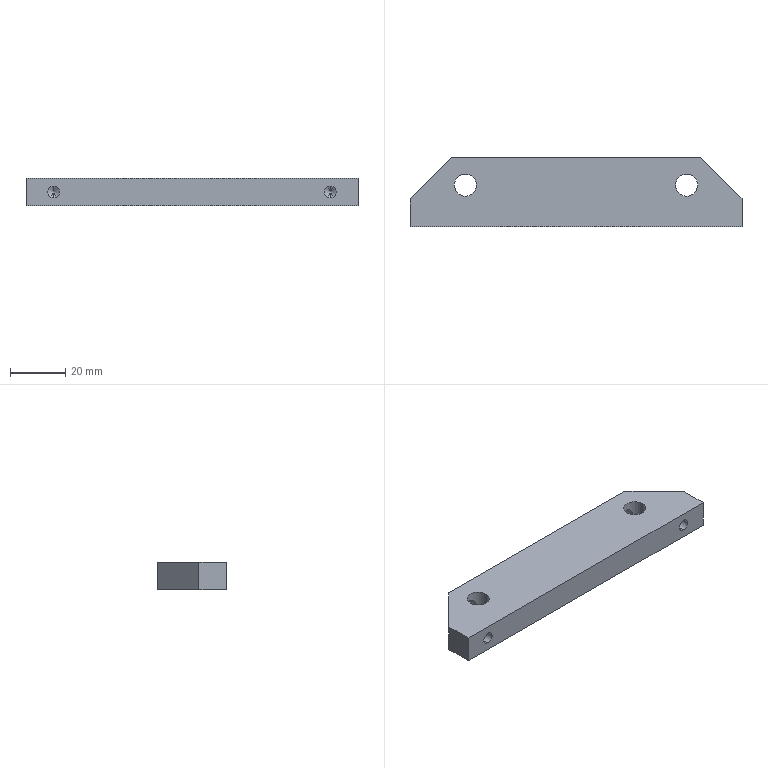Part | STEP file | CA-10-011Pusher Base_Default | 1 solid | 24 faces | box 120 x 25 x 10 mm | volume 26219 mm3 | cylinder 12 | plane 8 | cone 4 | commonest cylinder face diameters 4.2 x8 8 x4